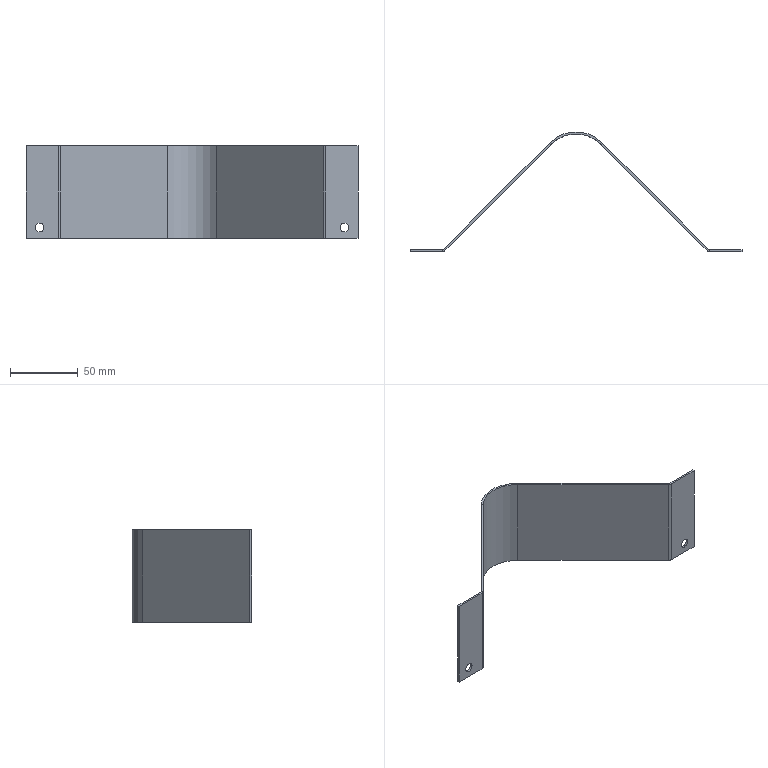Part | STEP file | Guard wheel drive wer2 | 1 solid | 32 faces | box 245 x 88.5 x 68.5 mm | volume 32228 mm3 | plane 24 | cylinder 8 | commonest cylinder face diameters 3 x2 6 x2 6.5 x2 51 x1 54 x1